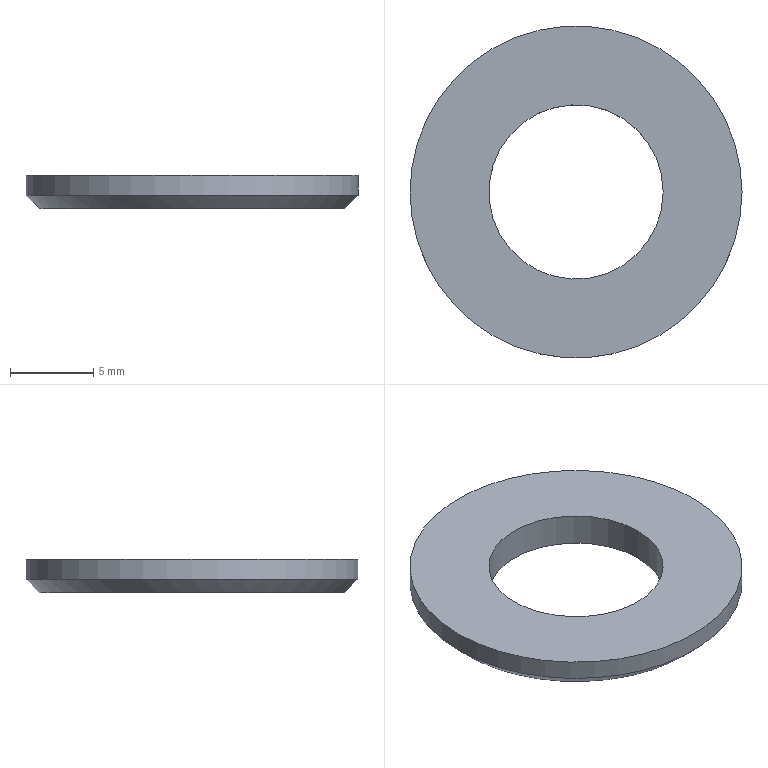Part | NX | features DATUM_CSYS 2, CHAMFER 1, EXTRUDE 1, SKETCH 1 | 1 solid | 5 faces | box 20 x 20 x 2 mm | volume 435.568 mm3 | cylinder 2 | plane 2 | cone 1 | commonest cylinder face diameters 10.5 x1 20 x1
STEP:
#1=CARTESIAN_POINT('',(10.,0.,0.8));
#2=VERTEX_POINT('',#1);
#3=CARTESIAN_POINT('',(0.,0.,0.8));
#4=DIRECTION('',(0.,0.,1.));
#5=DIRECTION('',(1.,0.,0.));
#6=AXIS2_PLACEMENT_3D('',#3,#4,#5);
#7=CIRCLE('',#6,10.);
#8=EDGE_CURVE('',#2,#2,#7,.T.);
#9=ORIENTED_EDGE('',*,*,#8,.T.);
#10=EDGE_LOOP('',(#9));
#11=FACE_BOUND('',#10,.T.);
#12=CARTESIAN_POINT('',(10.,0.,2.));
#13=VERTEX_POINT('',#12);
#14=CARTESIAN_POINT('',(0.,0.,2.));
#15=DIRECTION('',(0.,0.,1.));
#16=DIRECTION('',(1.,0.,0.));
#17=AXIS2_PLACEMENT_3D('',#14,#15,#16);
#18=CIRCLE('',#17,10.);
#19=EDGE_CURVE('',#13,#13,#18,.T.);
#20=ORIENTED_EDGE('',*,*,#19,.F.);
#21=EDGE_LOOP('',(#20));
#22=FACE_BOUND('',#21,.T.);
#23=CARTESIAN_POINT('',(0.,0.,2.));
#24=DIRECTION('',(0.,0.,-1.));
#25=DIRECTION('',(-1.,0.,0.));
#26=AXIS2_PLACEMENT_3D('',#23,#24,#25);
#27=CYLINDRICAL_SURFACE('',#26,10.);
#28=ADVANCED_FACE('',(#11,#22),#27,.T.);
#29=CARTESIAN_POINT('',(5.25,0.,2.));
#30=VERTEX_POINT('',#29);
#31=CARTESIAN_POINT('',(0.,0.,2.));
#32=DIRECTION('',(0.,0.,-1.));
#33=DIRECTION('',(1.,0.,0.));
#34=AXIS2_PLACEMENT_3D('',#31,#32,#33);
#35=CIRCLE('',#34,5.25);
#36=EDGE_CURVE('',#30,#30,#35,.T.);
#37=ORIENTED_EDGE('',*,*,#36,.F.);
#38=EDGE_LOOP('',(#37));
#39=FACE_BOUND('',#38,.T.);
#40=CARTESIAN_POINT('',(5.25,0.,0.));
#41=VERTEX_POINT('',#40);
#42=CARTESIAN_POINT('',(0.,0.,0.));
#43=DIRECTION('',(0.,0.,-1.));
#44=DIRECTION('',(1.,0.,0.));
#45=AXIS2_PLACEMENT_3D('',#42,#43,#44);
#46=CIRCLE('',#45,5.25);
#47=EDGE_CURVE('',#41,#41,#46,.T.);
#48=ORIENTED_EDGE('',*,*,#47,.T.);
#49=EDGE_LOOP('',(#48));
#50=FACE_BOUND('',#49,.T.);
#51=CARTESIAN_POINT('',(0.,0.,2.));
#52=DIRECTION('',(0.,0.,-1.));
#53=DIRECTION('',(-1.,0.,0.));
#54=AXIS2_PLACEMENT_3D('',#51,#52,#53);
#55=CYLINDRICAL_SURFACE('',#54,5.25);
#56=ADVANCED_FACE('',(#39,#50),#55,.F.);
#57=ORIENTED_EDGE('',*,*,#19,.T.);
#58=EDGE_LOOP('',(#57));
#59=FACE_BOUND('',#58,.T.);
#60=ORIENTED_EDGE('',*,*,#36,.T.);
#61=EDGE_LOOP('',(#60));
#62=FACE_BOUND('',#61,.T.);
#63=CARTESIAN_POINT('',(0.,0.,2.));
#64=DIRECTION('',(0.,0.,1.));
#65=DIRECTION('',(1.,0.,0.));
#66=AXIS2_PLACEMENT_3D('',#63,#64,#65);
#67=PLANE('',#66);
#68=ADVANCED_FACE('',(#59,#62),#67,.T.);
#69=CARTESIAN_POINT('',(9.2,0.,0.));
#70=VERTEX_POINT('',#69);
#71=CARTESIAN_POINT('',(0.,0.,0.));
#72=DIRECTION('',(0.,0.,1.));
#73=DIRECTION('',(1.,0.,0.));
#74=AXIS2_PLACEMENT_3D('',#71,#72,#73);
#75=CIRCLE('',#74,9.2);
#76=EDGE_CURVE('',#70,#70,#75,.F.);
#77=ORIENTED_EDGE('',*,*,#76,.T.);
#78=EDGE_LOOP('',(#77));
#79=FACE_BOUND('',#78,.T.);
#80=ORIENTED_EDGE('',*,*,#47,.F.);
#81=EDGE_LOOP('',(#80));
#82=FACE_BOUND('',#81,.T.);
#83=CARTESIAN_POINT('',(0.,0.,0.));
#84=DIRECTION('',(0.,0.,1.));
#85=DIRECTION('',(1.,0.,0.));
#86=AXIS2_PLACEMENT_3D('',#83,#84,#85);
#87=PLANE('',#86);
#88=ADVANCED_FACE('',(#79,#82),#87,.F.);
#89=ORIENTED_EDGE('',*,*,#76,.F.);
#90=EDGE_LOOP('',(#89));
#91=FACE_BOUND('',#90,.T.);
#92=ORIENTED_EDGE('',*,*,#8,.F.);
#93=EDGE_LOOP('',(#92));
#94=FACE_BOUND('',#93,.T.);
#95=CARTESIAN_POINT('',(0.,0.,0.8));
#96=DIRECTION('',(0.,0.,1.));
#97=DIRECTION('',(1.,0.,0.));
#98=AXIS2_PLACEMENT_3D('',#95,#96,#97);
#99=CONICAL_SURFACE('',#98,10.,0.7854);
#100=ADVANCED_FACE('',(#91,#94),#99,.T.);
#101=CLOSED_SHELL('',(#28,#56,#68,#88,#100));
#102=MANIFOLD_SOLID_BREP('',#101);
#103=(LENGTH_UNIT()NAMED_UNIT(*)SI_UNIT(.MILLI.,.METRE.));
#104=UNCERTAINTY_MEASURE_WITH_UNIT(LENGTH_MEASURE(0.00001),#103,'','');
#105=(NAMED_UNIT(*)PLANE_ANGLE_UNIT()SI_UNIT($,.RADIAN.));
#106=(NAMED_UNIT(*)SI_UNIT($,.STERADIAN.)SOLID_ANGLE_UNIT());
#107=(GEOMETRIC_REPRESENTATION_CONTEXT(3)GLOBAL_UNCERTAINTY_ASSIGNED_CONTEXT((#104))GLOBAL_UNIT_ASSIGNED_CONTEXT((#103,#105,#106))REPRESENTATION_CONTEXT('',''));
#108=ADVANCED_BREP_SHAPE_REPRESENTATION('',(#102),#107);